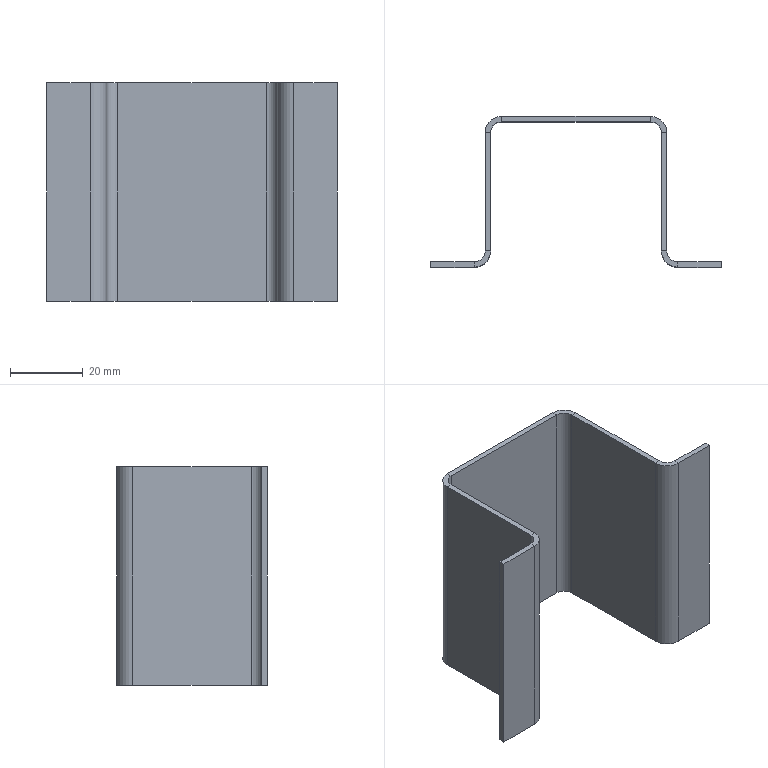Part | SolidWorks | features BaseBody 1 | 1 solid | 38 faces | box 80 x 41.5 x 60 mm | volume 13821 mm3 | plane 30 | cylinder 8 | commonest cylinder face diameters 6 x4 9 x4
STEP:
#1=CARTESIAN_POINT('',(68.,-1.5,-30.));
#2=VERTEX_POINT('',#1);
#3=CARTESIAN_POINT('',(80.,-1.5,-30.));
#4=VERTEX_POINT('',#3);
#5=CARTESIAN_POINT('',(65.,-1.5,-30.));
#6=DIRECTION('',(1.,0.,0.));
#7=VECTOR('',#6,1000.);
#8=LINE('',#5,#7);
#9=EDGE_CURVE('',#2,#4,#8,.T.);
#10=ORIENTED_EDGE('',*,*,#9,.F.);
#11=CARTESIAN_POINT('',(68.,0.,-30.));
#12=VERTEX_POINT('',#11);
#13=CARTESIAN_POINT('',(68.,-1.5,-30.));
#14=DIRECTION('',(0.,1.,0.));
#15=VECTOR('',#14,1000.);
#16=LINE('',#13,#15);
#17=EDGE_CURVE('',#2,#12,#16,.T.);
#18=ORIENTED_EDGE('',*,*,#17,.T.);
#19=CARTESIAN_POINT('',(80.,0.,-30.));
#20=VERTEX_POINT('',#19);
#21=CARTESIAN_POINT('',(65.,0.,-30.));
#22=DIRECTION('',(1.,0.,0.));
#23=VECTOR('',#22,1000.);
#24=LINE('',#21,#23);
#25=EDGE_CURVE('',#12,#20,#24,.T.);
#26=ORIENTED_EDGE('',*,*,#25,.T.);
#27=CARTESIAN_POINT('',(80.,0.,-30.));
#28=DIRECTION('',(0.,-1.,0.));
#29=VECTOR('',#28,1000.);
#30=LINE('',#27,#29);
#31=EDGE_CURVE('',#20,#4,#30,.T.);
#32=ORIENTED_EDGE('',*,*,#31,.T.);
#33=EDGE_LOOP('',(#10,#18,#26,#32));
#34=FACE_OUTER_BOUND('',#33,.T.);
#35=CARTESIAN_POINT('',(68.,3.,-30.));
#36=DIRECTION('',(0.,0.,-1.));
#37=DIRECTION('',(0.,-1.,0.));
#38=AXIS2_PLACEMENT_3D('',#35,#36,#37);
#39=PLANE('',#38);
#40=ADVANCED_FACE('',(#34),#39,.T.);
#41=CARTESIAN_POINT('',(0.,-1.5,30.));
#42=VERTEX_POINT('',#41);
#43=CARTESIAN_POINT('',(12.,-1.5,30.));
#44=VERTEX_POINT('',#43);
#45=CARTESIAN_POINT('',(0.,-1.5,30.));
#46=DIRECTION('',(1.,0.,0.));
#47=VECTOR('',#46,1000.);
#48=LINE('',#45,#47);
#49=EDGE_CURVE('',#42,#44,#48,.T.);
#50=ORIENTED_EDGE('',*,*,#49,.T.);
#51=CARTESIAN_POINT('',(12.,0.,30.));
#52=VERTEX_POINT('',#51);
#53=CARTESIAN_POINT('',(12.,-1.5,30.));
#54=DIRECTION('',(0.,1.,0.));
#55=VECTOR('',#54,1000.);
#56=LINE('',#53,#55);
#57=EDGE_CURVE('',#44,#52,#56,.T.);
#58=ORIENTED_EDGE('',*,*,#57,.T.);
#59=CARTESIAN_POINT('',(0.,0.,30.));
#60=VERTEX_POINT('',#59);
#61=CARTESIAN_POINT('',(0.,0.,30.));
#62=DIRECTION('',(1.,0.,0.));
#63=VECTOR('',#62,1000.);
#64=LINE('',#61,#63);
#65=EDGE_CURVE('',#60,#52,#64,.T.);
#66=ORIENTED_EDGE('',*,*,#65,.F.);
#67=CARTESIAN_POINT('',(0.,-1.5,30.));
#68=DIRECTION('',(0.,1.,0.));
#69=VECTOR('',#68,1000.);
#70=LINE('',#67,#69);
#71=EDGE_CURVE('',#42,#60,#70,.T.);
#72=ORIENTED_EDGE('',*,*,#71,.F.);
#73=EDGE_LOOP('',(#50,#58,#66,#72));
#74=FACE_OUTER_BOUND('',#73,.T.);
#75=CARTESIAN_POINT('',(68.,3.,30.));
#76=DIRECTION('',(0.,0.,-1.));
#77=DIRECTION('',(0.,-1.,0.));
#78=AXIS2_PLACEMENT_3D('',#75,#76,#77);
#79=PLANE('',#78);
#80=ADVANCED_FACE('',(#74),#79,.F.);
#81=CARTESIAN_POINT('',(63.5,3.,-30.));
#82=VERTEX_POINT('',#81);
#83=CARTESIAN_POINT('',(68.,3.,-30.));
#84=DIRECTION('',(0.,0.,1.));
#85=DIRECTION('',(1.,0.,0.));
#86=AXIS2_PLACEMENT_3D('',#83,#84,#85);
#87=CIRCLE('',#86,4.5);
#88=EDGE_CURVE('',#82,#2,#87,.T.);
#89=ORIENTED_EDGE('',*,*,#88,.T.);
#90=CARTESIAN_POINT('',(68.,-1.5,30.));
#91=VERTEX_POINT('',#90);
#92=CARTESIAN_POINT('',(68.,-1.5,30.));
#93=DIRECTION('',(0.,0.,-1.));
#94=VECTOR('',#93,1000.);
#95=LINE('',#92,#94);
#96=EDGE_CURVE('',#91,#2,#95,.T.);
#97=ORIENTED_EDGE('',*,*,#96,.F.);
#98=CARTESIAN_POINT('',(63.5,3.,30.));
#99=VERTEX_POINT('',#98);
#100=CARTESIAN_POINT('',(68.,3.,30.));
#101=DIRECTION('',(0.,0.,1.));
#102=DIRECTION('',(1.,0.,0.));
#103=AXIS2_PLACEMENT_3D('',#100,#101,#102);
#104=CIRCLE('',#103,4.5);
#105=EDGE_CURVE('',#99,#91,#104,.T.);
#106=ORIENTED_EDGE('',*,*,#105,.F.);
#107=CARTESIAN_POINT('',(63.5,3.,30.));
#108=DIRECTION('',(0.,0.,-1.));
#109=VECTOR('',#108,1000.);
#110=LINE('',#107,#109);
#111=EDGE_CURVE('',#99,#82,#110,.T.);
#112=ORIENTED_EDGE('',*,*,#111,.T.);
#113=EDGE_LOOP('',(#89,#97,#106,#112));
#114=FACE_OUTER_BOUND('',#113,.T.);
#115=CARTESIAN_POINT('',(68.,3.,30.));
#116=DIRECTION('',(0.,0.,-1.));
#117=DIRECTION('',(-1.,0.,0.));
#118=AXIS2_PLACEMENT_3D('',#115,#116,#117);
#119=CYLINDRICAL_SURFACE('',#118,4.5);
#120=ADVANCED_FACE('',(#114),#119,.T.);
#121=CARTESIAN_POINT('',(63.5,35.5,-30.));
#122=VERTEX_POINT('',#121);
#123=CARTESIAN_POINT('',(63.5,40.,-30.));
#124=DIRECTION('',(0.,-1.,0.));
#125=VECTOR('',#124,1000.);
#126=LINE('',#123,#125);
#127=EDGE_CURVE('',#122,#82,#126,.T.);
#128=ORIENTED_EDGE('',*,*,#127,.T.);
#129=ORIENTED_EDGE('',*,*,#111,.F.);
#130=CARTESIAN_POINT('',(63.5,35.5,30.));
#131=VERTEX_POINT('',#130);
#132=CARTESIAN_POINT('',(63.5,40.,30.));
#133=DIRECTION('',(0.,-1.,0.));
#134=VECTOR('',#133,1000.);
#135=LINE('',#132,#134);
#136=EDGE_CURVE('',#131,#99,#135,.T.);
#137=ORIENTED_EDGE('',*,*,#136,.F.);
#138=CARTESIAN_POINT('',(63.5,35.5,30.));
#139=DIRECTION('',(0.,0.,-1.));
#140=VECTOR('',#139,1000.);
#141=LINE('',#138,#140);
#142=EDGE_CURVE('',#131,#122,#141,.T.);
#143=ORIENTED_EDGE('',*,*,#142,.T.);
#144=EDGE_LOOP('',(#128,#129,#137,#143));
#145=FACE_OUTER_BOUND('',#144,.T.);
#146=CARTESIAN_POINT('',(63.5,40.,30.));
#147=DIRECTION('',(1.,0.,0.));
#148=DIRECTION('',(0.,1.,0.));
#149=AXIS2_PLACEMENT_3D('',#146,#147,#148);
#150=PLANE('',#149);
#151=ADVANCED_FACE('',(#145),#150,.F.);
#152=CARTESIAN_POINT('',(60.5,38.5,-30.));
#153=VERTEX_POINT('',#152);
#154=CARTESIAN_POINT('',(60.5,35.5,-30.));
#155=DIRECTION('',(0.,0.,-1.));
#156=DIRECTION('',(1.,0.,0.));
#157=AXIS2_PLACEMENT_3D('',#154,#155,#156);
#158=CIRCLE('',#157,3.);
#159=EDGE_CURVE('',#153,#122,#158,.T.);
#160=ORIENTED_EDGE('',*,*,#159,.T.);
#161=ORIENTED_EDGE('',*,*,#142,.F.);
#162=CARTESIAN_POINT('',(60.5,38.5,30.));
#163=VERTEX_POINT('',#162);
#164=CARTESIAN_POINT('',(60.5,35.5,30.));
#165=DIRECTION('',(0.,0.,-1.));
#166=DIRECTION('',(1.,0.,0.));
#167=AXIS2_PLACEMENT_3D('',#164,#165,#166);
#168=CIRCLE('',#167,3.);
#169=EDGE_CURVE('',#163,#131,#168,.T.);
#170=ORIENTED_EDGE('',*,*,#169,.F.);
#171=CARTESIAN_POINT('',(60.5,38.5,30.));
#172=DIRECTION('',(0.,0.,-1.));
#173=VECTOR('',#172,1000.);
#174=LINE('',#171,#173);
#175=EDGE_CURVE('',#163,#153,#174,.T.);
#176=ORIENTED_EDGE('',*,*,#175,.T.);
#177=EDGE_LOOP('',(#160,#161,#170,#176));
#178=FACE_OUTER_BOUND('',#177,.T.);
#179=CARTESIAN_POINT('',(60.5,35.5,30.));
#180=DIRECTION('',(0.,0.,-1.));
#181=DIRECTION('',(-1.,0.,0.));
#182=AXIS2_PLACEMENT_3D('',#179,#180,#181);
#183=CYLINDRICAL_SURFACE('',#182,3.);
#184=ADVANCED_FACE('',(#178),#183,.F.);
#185=CARTESIAN_POINT('',(19.5,38.5,-30.));
#186=VERTEX_POINT('',#185);
#187=CARTESIAN_POINT('',(15.,38.5,-30.));
#188=DIRECTION('',(1.,0.,0.));
#189=VECTOR('',#188,1000.);
#190=LINE('',#187,#189);
#191=EDGE_CURVE('',#186,#153,#190,.T.);
#192=ORIENTED_EDGE('',*,*,#191,.T.);
#193=ORIENTED_EDGE('',*,*,#175,.F.);
#194=CARTESIAN_POINT('',(19.5,38.5,30.));
#195=VERTEX_POINT('',#194);
#196=CARTESIAN_POINT('',(15.,38.5,30.));
#197=DIRECTION('',(1.,0.,0.));
#198=VECTOR('',#197,1000.);
#199=LINE('',#196,#198);
#200=EDGE_CURVE('',#195,#163,#199,.T.);
#201=ORIENTED_EDGE('',*,*,#200,.F.);
#202=CARTESIAN_POINT('',(19.5,38.5,30.));
#203=DIRECTION('',(0.,0.,-1.));
#204=VECTOR('',#203,1000.);
#205=LINE('',#202,#204);
#206=EDGE_CURVE('',#195,#186,#205,.T.);
#207=ORIENTED_EDGE('',*,*,#206,.T.);
#208=EDGE_LOOP('',(#192,#193,#201,#207));
#209=FACE_OUTER_BOUND('',#208,.T.);
#210=CARTESIAN_POINT('',(15.,38.5,30.));
#211=DIRECTION('',(0.,1.,0.));
#212=DIRECTION('',(1.,0.,0.));
#213=AXIS2_PLACEMENT_3D('',#210,#211,#212);
#214=PLANE('',#213);
#215=ADVANCED_FACE('',(#209),#214,.F.);
#216=CARTESIAN_POINT('',(16.5,35.5,-30.));
#217=VERTEX_POINT('',#216);
#218=CARTESIAN_POINT('',(19.5,35.5,-30.));
#219=DIRECTION('',(0.,0.,-1.));
#220=DIRECTION('',(1.,0.,0.));
#221=AXIS2_PLACEMENT_3D('',#218,#219,#220);
#222=CIRCLE('',#221,3.);
#223=EDGE_CURVE('',#217,#186,#222,.T.);
#224=ORIENTED_EDGE('',*,*,#223,.T.);
#225=ORIENTED_EDGE('',*,*,#206,.F.);
#226=CARTESIAN_POINT('',(16.5,35.5,30.));
#227=VERTEX_POINT('',#226);
#228=CARTESIAN_POINT('',(19.5,35.5,30.));
#229=DIRECTION('',(0.,0.,-1.));
#230=DIRECTION('',(1.,0.,0.));
#231=AXIS2_PLACEMENT_3D('',#228,#229,#230);
#232=CIRCLE('',#231,3.);
#233=EDGE_CURVE('',#227,#195,#232,.T.);
#234=ORIENTED_EDGE('',*,*,#233,.F.);
#235=CARTESIAN_POINT('',(16.5,35.5,30.));
#236=DIRECTION('',(0.,0.,-1.));
#237=VECTOR('',#236,1000.);
#238=LINE('',#235,#237);
#239=EDGE_CURVE('',#227,#217,#238,.T.);
#240=ORIENTED_EDGE('',*,*,#239,.T.);
#241=EDGE_LOOP('',(#224,#225,#234,#240));
#242=FACE_OUTER_BOUND('',#241,.T.);
#243=CARTESIAN_POINT('',(19.5,35.5,30.));
#244=DIRECTION('',(0.,0.,-1.));
#245=DIRECTION('',(-1.,0.,0.));
#246=AXIS2_PLACEMENT_3D('',#243,#244,#245);
#247=CYLINDRICAL_SURFACE('',#246,3.);
#248=ADVANCED_FACE('',(#242),#247,.F.);
#249=CARTESIAN_POINT('',(16.5,3.,-30.));
#250=VERTEX_POINT('',#249);
#251=CARTESIAN_POINT('',(16.5,0.,-30.));
#252=DIRECTION('',(0.,1.,0.));
#253=VECTOR('',#252,1000.);
#254=LINE('',#251,#253);
#255=EDGE_CURVE('',#250,#217,#254,.T.);
#256=ORIENTED_EDGE('',*,*,#255,.T.);
#257=ORIENTED_EDGE('',*,*,#239,.F.);
#258=CARTESIAN_POINT('',(16.5,3.,30.));
#259=VERTEX_POINT('',#258);
#260=CARTESIAN_POINT('',(16.5,0.,30.));
#261=DIRECTION('',(0.,1.,0.));
#262=VECTOR('',#261,1000.);
#263=LINE('',#260,#262);
#264=EDGE_CURVE('',#259,#227,#263,.T.);
#265=ORIENTED_EDGE('',*,*,#264,.F.);
#266=CARTESIAN_POINT('',(16.5,3.,30.));
#267=DIRECTION('',(0.,0.,-1.));
#268=VECTOR('',#267,1000.);
#269=LINE('',#266,#268);
#270=EDGE_CURVE('',#259,#250,#269,.T.);
#271=ORIENTED_EDGE('',*,*,#270,.T.);
#272=EDGE_LOOP('',(#256,#257,#265,#271));
#273=FACE_OUTER_BOUND('',#272,.T.);
#274=CARTESIAN_POINT('',(16.5,0.,30.));
#275=DIRECTION('',(-1.,0.,0.));
#276=DIRECTION('',(0.,0.,1.));
#277=AXIS2_PLACEMENT_3D('',#274,#275,#276);
#278=PLANE('',#277);
#279=ADVANCED_FACE('',(#273),#278,.F.);
#280=CARTESIAN_POINT('',(12.,-1.5,-30.));
#281=VERTEX_POINT('',#280);
#282=CARTESIAN_POINT('',(12.,3.,-30.));
#283=DIRECTION('',(0.,0.,1.));
#284=DIRECTION('',(1.,0.,0.));
#285=AXIS2_PLACEMENT_3D('',#282,#283,#284);
#286=CIRCLE('',#285,4.5);
#287=EDGE_CURVE('',#281,#250,#286,.T.);
#288=ORIENTED_EDGE('',*,*,#287,.T.);
#289=ORIENTED_EDGE('',*,*,#270,.F.);
#290=CARTESIAN_POINT('',(12.,3.,30.));
#291=DIRECTION('',(0.,0.,1.));
#292=DIRECTION('',(1.,0.,0.));
#293=AXIS2_PLACEMENT_3D('',#290,#291,#292);
#294=CIRCLE('',#293,4.5);
#295=EDGE_CURVE('',#44,#259,#294,.T.);
#296=ORIENTED_EDGE('',*,*,#295,.F.);
#297=CARTESIAN_POINT('',(12.,-1.5,30.));
#298=DIRECTION('',(0.,0.,-1.));
#299=VECTOR('',#298,1000.);
#300=LINE('',#297,#299);
#301=EDGE_CURVE('',#44,#281,#300,.T.);
#302=ORIENTED_EDGE('',*,*,#301,.T.);
#303=EDGE_LOOP('',(#288,#289,#296,#302));
#304=FACE_OUTER_BOUND('',#303,.T.);
#305=CARTESIAN_POINT('',(12.,3.,30.));
#306=DIRECTION('',(0.,0.,-1.));
#307=DIRECTION('',(-1.,0.,0.));
#308=AXIS2_PLACEMENT_3D('',#305,#306,#307);
#309=CYLINDRICAL_SURFACE('',#308,4.5);
#310=ADVANCED_FACE('',(#304),#309,.T.);
#311=CARTESIAN_POINT('',(0.,-1.5,-30.));
#312=VERTEX_POINT('',#311);
#313=CARTESIAN_POINT('',(0.,-1.5,-30.));
#314=DIRECTION('',(1.,0.,0.));
#315=VECTOR('',#314,1000.);
#316=LINE('',#313,#315);
#317=EDGE_CURVE('',#312,#281,#316,.T.);
#318=ORIENTED_EDGE('',*,*,#317,.T.);
#319=ORIENTED_EDGE('',*,*,#301,.F.);
#320=ORIENTED_EDGE('',*,*,#49,.F.);
#321=CARTESIAN_POINT('',(0.,-1.5,30.));
#322=DIRECTION('',(0.,0.,-1.));
#323=VECTOR('',#322,1000.);
#324=LINE('',#321,#323);
#325=EDGE_CURVE('',#42,#312,#324,.T.);
#326=ORIENTED_EDGE('',*,*,#325,.T.);
#327=EDGE_LOOP('',(#318,#319,#320,#326));
#328=FACE_OUTER_BOUND('',#327,.T.);
#329=CARTESIAN_POINT('',(0.,-1.5,30.));
#330=DIRECTION('',(0.,1.,0.));
#331=DIRECTION('',(1.,0.,0.));
#332=AXIS2_PLACEMENT_3D('',#329,#330,#331);
#333=PLANE('',#332);
#334=ADVANCED_FACE('',(#328),#333,.F.);
#335=CARTESIAN_POINT('',(0.,0.,-30.));
#336=VERTEX_POINT('',#335);
#337=CARTESIAN_POINT('',(0.,-1.5,-30.));
#338=DIRECTION('',(0.,1.,0.));
#339=VECTOR('',#338,1000.);
#340=LINE('',#337,#339);
#341=EDGE_CURVE('',#312,#336,#340,.T.);
#342=ORIENTED_EDGE('',*,*,#341,.F.);
#343=ORIENTED_EDGE('',*,*,#325,.F.);
#344=ORIENTED_EDGE('',*,*,#71,.T.);
#345=CARTESIAN_POINT('',(0.,0.,30.));
#346=DIRECTION('',(0.,0.,-1.));
#347=VECTOR('',#346,1000.);
#348=LINE('',#345,#347);
#349=EDGE_CURVE('',#60,#336,#348,.T.);
#350=ORIENTED_EDGE('',*,*,#349,.T.);
#351=EDGE_LOOP('',(#342,#343,#344,#350));
#352=FACE_OUTER_BOUND('',#351,.T.);
#353=CARTESIAN_POINT('',(0.,-1.5,30.));
#354=DIRECTION('',(-1.,0.,0.));
#355=DIRECTION('',(0.,0.,1.));
#356=AXIS2_PLACEMENT_3D('',#353,#354,#355);
#357=PLANE('',#356);
#358=ADVANCED_FACE('',(#352),#357,.T.);
#359=CARTESIAN_POINT('',(12.,0.,-30.));
#360=VERTEX_POINT('',#359);
#361=CARTESIAN_POINT('',(0.,0.,-30.));
#362=DIRECTION('',(1.,0.,0.));
#363=VECTOR('',#362,1000.);
#364=LINE('',#361,#363);
#365=EDGE_CURVE('',#336,#360,#364,.T.);
#366=ORIENTED_EDGE('',*,*,#365,.F.);
#367=ORIENTED_EDGE('',*,*,#349,.F.);
#368=ORIENTED_EDGE('',*,*,#65,.T.);
#369=CARTESIAN_POINT('',(12.,0.,30.));
#370=DIRECTION('',(0.,0.,-1.));
#371=VECTOR('',#370,1000.);
#372=LINE('',#369,#371);
#373=EDGE_CURVE('',#52,#360,#372,.T.);
#374=ORIENTED_EDGE('',*,*,#373,.T.);
#375=EDGE_LOOP('',(#366,#367,#368,#374));
#376=FACE_OUTER_BOUND('',#375,.T.);
#377=CARTESIAN_POINT('',(0.,0.,30.));
#378=DIRECTION('',(0.,1.,0.));
#379=DIRECTION('',(1.,0.,0.));
#380=AXIS2_PLACEMENT_3D('',#377,#378,#379);
#381=PLANE('',#380);
#382=ADVANCED_FACE('',(#376),#381,.T.);
#383=CARTESIAN_POINT('',(15.,3.,-30.));
#384=VERTEX_POINT('',#383);
#385=CARTESIAN_POINT('',(12.,3.,-30.));
#386=DIRECTION('',(0.,0.,1.));
#387=DIRECTION('',(-1.,0.,0.));
#388=AXIS2_PLACEMENT_3D('',#385,#386,#387);
#389=CIRCLE('',#388,3.);
#390=EDGE_CURVE('',#360,#384,#389,.T.);
#391=ORIENTED_EDGE('',*,*,#390,.F.);
#392=ORIENTED_EDGE('',*,*,#373,.F.);
#393=CARTESIAN_POINT('',(15.,3.,30.));
#394=VERTEX_POINT('',#393);
#395=CARTESIAN_POINT('',(12.,3.,30.));
#396=DIRECTION('',(0.,0.,1.));
#397=DIRECTION('',(-1.,0.,0.));
#398=AXIS2_PLACEMENT_3D('',#395,#396,#397);
#399=CIRCLE('',#398,3.);
#400=EDGE_CURVE('',#52,#394,#399,.T.);
#401=ORIENTED_EDGE('',*,*,#400,.T.);
#402=CARTESIAN_POINT('',(15.,3.,30.));
#403=DIRECTION('',(0.,0.,-1.));
#404=VECTOR('',#403,1000.);
#405=LINE('',#402,#404);
#406=EDGE_CURVE('',#394,#384,#405,.T.);
#407=ORIENTED_EDGE('',*,*,#406,.T.);
#408=EDGE_LOOP('',(#391,#392,#401,#407));
#409=FACE_OUTER_BOUND('',#408,.T.);
#410=CARTESIAN_POINT('',(12.,3.,30.));
#411=DIRECTION('',(0.,0.,-1.));
#412=DIRECTION('',(-1.,0.,0.));
#413=AXIS2_PLACEMENT_3D('',#410,#411,#412);
#414=CYLINDRICAL_SURFACE('',#413,3.);
#415=ADVANCED_FACE('',(#409),#414,.F.);
#416=CARTESIAN_POINT('',(15.,35.5,-30.));
#417=VERTEX_POINT('',#416);
#418=CARTESIAN_POINT('',(15.,0.,-30.));
#419=DIRECTION('',(0.,1.,0.));
#420=VECTOR('',#419,1000.);
#421=LINE('',#418,#420);
#422=EDGE_CURVE('',#384,#417,#421,.T.);
#423=ORIENTED_EDGE('',*,*,#422,.F.);
#424=ORIENTED_EDGE('',*,*,#406,.F.);
#425=CARTESIAN_POINT('',(15.,35.5,30.));
#426=VERTEX_POINT('',#425);
#427=CARTESIAN_POINT('',(15.,0.,30.));
#428=DIRECTION('',(0.,1.,0.));
#429=VECTOR('',#428,1000.);
#430=LINE('',#427,#429);
#431=EDGE_CURVE('',#394,#426,#430,.T.);
#432=ORIENTED_EDGE('',*,*,#431,.T.);
#433=CARTESIAN_POINT('',(15.,35.5,30.));
#434=DIRECTION('',(0.,0.,-1.));
#435=VECTOR('',#434,1000.);
#436=LINE('',#433,#435);
#437=EDGE_CURVE('',#426,#417,#436,.T.);
#438=ORIENTED_EDGE('',*,*,#437,.T.);
#439=EDGE_LOOP('',(#423,#424,#432,#438));
#440=FACE_OUTER_BOUND('',#439,.T.);
#441=CARTESIAN_POINT('',(15.,0.,30.));
#442=DIRECTION('',(-1.,0.,0.));
#443=DIRECTION('',(0.,0.,1.));
#444=AXIS2_PLACEMENT_3D('',#441,#442,#443);
#445=PLANE('',#444);
#446=ADVANCED_FACE('',(#440),#445,.T.);
#447=CARTESIAN_POINT('',(19.5,40.,-30.));
#448=VERTEX_POINT('',#447);
#449=CARTESIAN_POINT('',(19.5,35.5,-30.));
#450=DIRECTION('',(0.,0.,-1.));
#451=DIRECTION('',(1.,0.,0.));
#452=AXIS2_PLACEMENT_3D('',#449,#450,#451);
#453=CIRCLE('',#452,4.5);
#454=EDGE_CURVE('',#417,#448,#453,.T.);
#455=ORIENTED_EDGE('',*,*,#454,.F.);
#456=ORIENTED_EDGE('',*,*,#437,.F.);
#457=CARTESIAN_POINT('',(19.5,40.,30.));
#458=VERTEX_POINT('',#457);
#459=CARTESIAN_POINT('',(19.5,35.5,30.));
#460=DIRECTION('',(0.,0.,-1.));
#461=DIRECTION('',(1.,0.,0.));
#462=AXIS2_PLACEMENT_3D('',#459,#460,#461);
#463=CIRCLE('',#462,4.5);
#464=EDGE_CURVE('',#426,#458,#463,.T.);
#465=ORIENTED_EDGE('',*,*,#464,.T.);
#466=CARTESIAN_POINT('',(19.5,40.,30.));
#467=DIRECTION('',(0.,0.,-1.));
#468=VECTOR('',#467,1000.);
#469=LINE('',#466,#468);
#470=EDGE_CURVE('',#458,#448,#469,.T.);
#471=ORIENTED_EDGE('',*,*,#470,.T.);
#472=EDGE_LOOP('',(#455,#456,#465,#471));
#473=FACE_OUTER_BOUND('',#472,.T.);
#474=CARTESIAN_POINT('',(19.5,35.5,30.));
#475=DIRECTION('',(0.,0.,-1.));
#476=DIRECTION('',(-1.,0.,0.));
#477=AXIS2_PLACEMENT_3D('',#474,#475,#476);
#478=CYLINDRICAL_SURFACE('',#477,4.5);
#479=ADVANCED_FACE('',(#473),#478,.T.);
#480=CARTESIAN_POINT('',(60.5,40.,-30.));
#481=VERTEX_POINT('',#480);
#482=CARTESIAN_POINT('',(15.,40.,-30.));
#483=DIRECTION('',(1.,0.,0.));
#484=VECTOR('',#483,1000.);
#485=LINE('',#482,#484);
#486=EDGE_CURVE('',#448,#481,#485,.T.);
#487=ORIENTED_EDGE('',*,*,#486,.F.);
#488=ORIENTED_EDGE('',*,*,#470,.F.);
#489=CARTESIAN_POINT('',(60.5,40.,30.));
#490=VERTEX_POINT('',#489);
#491=CARTESIAN_POINT('',(15.,40.,30.));
#492=DIRECTION('',(1.,0.,0.));
#493=VECTOR('',#492,1000.);
#494=LINE('',#491,#493);
#495=EDGE_CURVE('',#458,#490,#494,.T.);
#496=ORIENTED_EDGE('',*,*,#495,.T.);
#497=CARTESIAN_POINT('',(60.5,40.,30.));
#498=DIRECTION('',(0.,0.,-1.));
#499=VECTOR('',#498,1000.);
#500=LINE('',#497,#499);
#501=EDGE_CURVE('',#490,#481,#500,.T.);
#502=ORIENTED_EDGE('',*,*,#501,.T.);
#503=EDGE_LOOP('',(#487,#488,#496,#502));
#504=FACE_OUTER_BOUND('',#503,.T.);
#505=CARTESIAN_POINT('',(15.,40.,30.));
#506=DIRECTION('',(0.,1.,0.));
#507=DIRECTION('',(1.,0.,0.));
#508=AXIS2_PLACEMENT_3D('',#505,#506,#507);
#509=PLANE('',#508);
#510=ADVANCED_FACE('',(#504),#509,.T.);
#511=CARTESIAN_POINT('',(65.,35.5,-30.));
#512=VERTEX_POINT('',#511);
#513=CARTESIAN_POINT('',(60.5,35.5,-30.));
#514=DIRECTION('',(0.,0.,-1.));
#515=DIRECTION('',(1.,0.,0.));
#516=AXIS2_PLACEMENT_3D('',#513,#514,#515);
#517=CIRCLE('',#516,4.5);
#518=EDGE_CURVE('',#481,#512,#517,.T.);
#519=ORIENTED_EDGE('',*,*,#518,.F.);
#520=ORIENTED_EDGE('',*,*,#501,.F.);
#521=CARTESIAN_POINT('',(65.,35.5,30.));
#522=VERTEX_POINT('',#521);
#523=CARTESIAN_POINT('',(60.5,35.5,30.));
#524=DIRECTION('',(0.,0.,-1.));
#525=DIRECTION('',(1.,0.,0.));
#526=AXIS2_PLACEMENT_3D('',#523,#524,#525);
#527=CIRCLE('',#526,4.5);
#528=EDGE_CURVE('',#490,#522,#527,.T.);
#529=ORIENTED_EDGE('',*,*,#528,.T.);
#530=CARTESIAN_POINT('',(65.,35.5,30.));
#531=DIRECTION('',(0.,0.,-1.));
#532=VECTOR('',#531,1000.);
#533=LINE('',#530,#532);
#534=EDGE_CURVE('',#522,#512,#533,.T.);
#535=ORIENTED_EDGE('',*,*,#534,.T.);
#536=EDGE_LOOP('',(#519,#520,#529,#535));
#537=FACE_OUTER_BOUND('',#536,.T.);
#538=CARTESIAN_POINT('',(60.5,35.5,30.));
#539=DIRECTION('',(0.,0.,-1.));
#540=DIRECTION('',(-1.,0.,0.));
#541=AXIS2_PLACEMENT_3D('',#538,#539,#540);
#542=CYLINDRICAL_SURFACE('',#541,4.5);
#543=ADVANCED_FACE('',(#537),#542,.T.);
#544=CARTESIAN_POINT('',(65.,3.,-30.));
#545=VERTEX_POINT('',#544);
#546=CARTESIAN_POINT('',(65.,40.,-30.));
#547=DIRECTION('',(0.,-1.,0.));
#548=VECTOR('',#547,1000.);
#549=LINE('',#546,#548);
#550=EDGE_CURVE('',#512,#545,#549,.T.);
#551=ORIENTED_EDGE('',*,*,#550,.F.);
#552=ORIENTED_EDGE('',*,*,#534,.F.);
#553=CARTESIAN_POINT('',(65.,3.,30.));
#554=VERTEX_POINT('',#553);
#555=CARTESIAN_POINT('',(65.,40.,30.));
#556=DIRECTION('',(0.,-1.,0.));
#557=VECTOR('',#556,1000.);
#558=LINE('',#555,#557);
#559=EDGE_CURVE('',#522,#554,#558,.T.);
#560=ORIENTED_EDGE('',*,*,#559,.T.);
#561=CARTESIAN_POINT('',(65.,3.,30.));
#562=DIRECTION('',(0.,0.,-1.));
#563=VECTOR('',#562,1000.);
#564=LINE('',#561,#563);
#565=EDGE_CURVE('',#554,#545,#564,.T.);
#566=ORIENTED_EDGE('',*,*,#565,.T.);
#567=EDGE_LOOP('',(#551,#552,#560,#566));
#568=FACE_OUTER_BOUND('',#567,.T.);
#569=CARTESIAN_POINT('',(65.,40.,30.));
#570=DIRECTION('',(1.,0.,0.));
#571=DIRECTION('',(0.,1.,0.));
#572=AXIS2_PLACEMENT_3D('',#569,#570,#571);
#573=PLANE('',#572);
#574=ADVANCED_FACE('',(#568),#573,.T.);
#575=CARTESIAN_POINT('',(68.,3.,-30.));
#576=DIRECTION('',(0.,0.,1.));
#577=DIRECTION('',(-1.,0.,0.));
#578=AXIS2_PLACEMENT_3D('',#575,#576,#577);
#579=CIRCLE('',#578,3.);
#580=EDGE_CURVE('',#545,#12,#579,.T.);
#581=ORIENTED_EDGE('',*,*,#580,.F.);
#582=ORIENTED_EDGE('',*,*,#565,.F.);
#583=CARTESIAN_POINT('',(68.,0.,30.));
#584=VERTEX_POINT('',#583);
#585=CARTESIAN_POINT('',(68.,3.,30.));
#586=DIRECTION('',(0.,0.,1.));
#587=DIRECTION('',(-1.,0.,0.));
#588=AXIS2_PLACEMENT_3D('',#585,#586,#587);
#589=CIRCLE('',#588,3.);
#590=EDGE_CURVE('',#554,#584,#589,.T.);
#591=ORIENTED_EDGE('',*,*,#590,.T.);
#592=CARTESIAN_POINT('',(68.,0.,30.));
#593=DIRECTION('',(0.,0.,-1.));
#594=VECTOR('',#593,1000.);
#595=LINE('',#592,#594);
#596=EDGE_CURVE('',#584,#12,#595,.T.);
#597=ORIENTED_EDGE('',*,*,#596,.T.);
#598=EDGE_LOOP('',(#581,#582,#591,#597));
#599=FACE_OUTER_BOUND('',#598,.T.);
#600=CARTESIAN_POINT('',(68.,3.,30.));
#601=DIRECTION('',(0.,0.,-1.));
#602=DIRECTION('',(-1.,0.,0.));
#603=AXIS2_PLACEMENT_3D('',#600,#601,#602);
#604=CYLINDRICAL_SURFACE('',#603,3.);
#605=ADVANCED_FACE('',(#599),#604,.F.);
#606=ORIENTED_EDGE('',*,*,#25,.F.);
#607=ORIENTED_EDGE('',*,*,#596,.F.);
#608=CARTESIAN_POINT('',(80.,0.,30.));
#609=VERTEX_POINT('',#608);
#610=CARTESIAN_POINT('',(65.,0.,30.));
#611=DIRECTION('',(1.,0.,0.));
#612=VECTOR('',#611,1000.);
#613=LINE('',#610,#612);
#614=EDGE_CURVE('',#584,#609,#613,.T.);
#615=ORIENTED_EDGE('',*,*,#614,.T.);
#616=CARTESIAN_POINT('',(80.,0.,30.));
#617=DIRECTION('',(0.,0.,-1.));
#618=VECTOR('',#617,1000.);
#619=LINE('',#616,#618);
#620=EDGE_CURVE('',#609,#20,#619,.T.);
#621=ORIENTED_EDGE('',*,*,#620,.T.);
#622=EDGE_LOOP('',(#606,#607,#615,#621));
#623=FACE_OUTER_BOUND('',#622,.T.);
#624=CARTESIAN_POINT('',(65.,0.,30.));
#625=DIRECTION('',(0.,1.,0.));
#626=DIRECTION('',(1.,0.,0.));
#627=AXIS2_PLACEMENT_3D('',#624,#625,#626);
#628=PLANE('',#627);
#629=ADVANCED_FACE('',(#623),#628,.T.);
#630=ORIENTED_EDGE('',*,*,#31,.F.);
#631=ORIENTED_EDGE('',*,*,#620,.F.);
#632=CARTESIAN_POINT('',(80.,-1.5,30.));
#633=VERTEX_POINT('',#632);
#634=CARTESIAN_POINT('',(80.,0.,30.));
#635=DIRECTION('',(0.,-1.,0.));
#636=VECTOR('',#635,1000.);
#637=LINE('',#634,#636);
#638=EDGE_CURVE('',#609,#633,#637,.T.);
#639=ORIENTED_EDGE('',*,*,#638,.T.);
#640=CARTESIAN_POINT('',(80.,-1.5,30.));
#641=DIRECTION('',(0.,0.,-1.));
#642=VECTOR('',#641,1000.);
#643=LINE('',#640,#642);
#644=EDGE_CURVE('',#633,#4,#643,.T.);
#645=ORIENTED_EDGE('',*,*,#644,.T.);
#646=EDGE_LOOP('',(#630,#631,#639,#645));
#647=FACE_OUTER_BOUND('',#646,.T.);
#648=CARTESIAN_POINT('',(80.,0.,30.));
#649=DIRECTION('',(1.,0.,0.));
#650=DIRECTION('',(0.,1.,0.));
#651=AXIS2_PLACEMENT_3D('',#648,#649,#650);
#652=PLANE('',#651);
#653=ADVANCED_FACE('',(#647),#652,.T.);
#654=ORIENTED_EDGE('',*,*,#9,.T.);
#655=ORIENTED_EDGE('',*,*,#644,.F.);
#656=CARTESIAN_POINT('',(65.,-1.5,30.));
#657=DIRECTION('',(1.,0.,0.));
#658=VECTOR('',#657,1000.);
#659=LINE('',#656,#658);
#660=EDGE_CURVE('',#91,#633,#659,.T.);
#661=ORIENTED_EDGE('',*,*,#660,.F.);
#662=ORIENTED_EDGE('',*,*,#96,.T.);
#663=EDGE_LOOP('',(#654,#655,#661,#662));
#664=FACE_OUTER_BOUND('',#663,.T.);
#665=CARTESIAN_POINT('',(65.,-1.5,30.));
#666=DIRECTION('',(0.,1.,0.));
#667=DIRECTION('',(1.,0.,0.));
#668=AXIS2_PLACEMENT_3D('',#665,#666,#667);
#669=PLANE('',#668);
#670=ADVANCED_FACE('',(#664),#669,.F.);
#671=ORIENTED_EDGE('',*,*,#550,.T.);
#672=CARTESIAN_POINT('',(65.,3.,-30.));
#673=DIRECTION('',(-1.,0.,0.));
#674=VECTOR('',#673,1000.);
#675=LINE('',#672,#674);
#676=EDGE_CURVE('',#545,#82,#675,.T.);
#677=ORIENTED_EDGE('',*,*,#676,.T.);
#678=ORIENTED_EDGE('',*,*,#127,.F.);
#679=CARTESIAN_POINT('',(63.5,35.5,-30.));
#680=DIRECTION('',(1.,0.,0.));
#681=VECTOR('',#680,1000.);
#682=LINE('',#679,#681);
#683=EDGE_CURVE('',#122,#512,#682,.T.);
#684=ORIENTED_EDGE('',*,*,#683,.T.);
#685=EDGE_LOOP('',(#671,#677,#678,#684));
#686=FACE_OUTER_BOUND('',#685,.T.);
#687=CARTESIAN_POINT('',(68.,-1.5,-30.));
#688=DIRECTION('',(0.,0.,-1.));
#689=DIRECTION('',(0.,-1.,0.));
#690=AXIS2_PLACEMENT_3D('',#687,#688,#689);
#691=PLANE('',#690);
#692=ADVANCED_FACE('',(#686),#691,.T.);
#693=ORIENTED_EDGE('',*,*,#676,.F.);
#694=ORIENTED_EDGE('',*,*,#580,.T.);
#695=ORIENTED_EDGE('',*,*,#17,.F.);
#696=ORIENTED_EDGE('',*,*,#88,.F.);
#697=EDGE_LOOP('',(#693,#694,#695,#696));
#698=FACE_OUTER_BOUND('',#697,.T.);
#699=CARTESIAN_POINT('',(65.,3.,-30.));
#700=DIRECTION('',(0.,0.,-1.));
#701=DIRECTION('',(0.,-1.,0.));
#702=AXIS2_PLACEMENT_3D('',#699,#700,#701);
#703=PLANE('',#702);
#704=ADVANCED_FACE('',(#698),#703,.T.);
#705=ORIENTED_EDGE('',*,*,#614,.F.);
#706=CARTESIAN_POINT('',(68.,0.,30.));
#707=DIRECTION('',(0.,-1.,0.));
#708=VECTOR('',#707,1000.);
#709=LINE('',#706,#708);
#710=EDGE_CURVE('',#584,#91,#709,.T.);
#711=ORIENTED_EDGE('',*,*,#710,.T.);
#712=ORIENTED_EDGE('',*,*,#660,.T.);
#713=ORIENTED_EDGE('',*,*,#638,.F.);
#714=EDGE_LOOP('',(#705,#711,#712,#713));
#715=FACE_OUTER_BOUND('',#714,.T.);
#716=CARTESIAN_POINT('',(63.5,3.,30.));
#717=DIRECTION('',(0.,0.,1.));
#718=DIRECTION('',(1.,0.,0.));
#719=AXIS2_PLACEMENT_3D('',#716,#717,#718);
#720=PLANE('',#719);
#721=ADVANCED_FACE('',(#715),#720,.T.);
#722=ORIENTED_EDGE('',*,*,#710,.F.);
#723=ORIENTED_EDGE('',*,*,#590,.F.);
#724=CARTESIAN_POINT('',(63.5,3.,30.));
#725=DIRECTION('',(1.,0.,0.));
#726=VECTOR('',#725,1000.);
#727=LINE('',#724,#726);
#728=EDGE_CURVE('',#99,#554,#727,.T.);
#729=ORIENTED_EDGE('',*,*,#728,.F.);
#730=ORIENTED_EDGE('',*,*,#105,.T.);
#731=EDGE_LOOP('',(#722,#723,#729,#730));
#732=FACE_OUTER_BOUND('',#731,.T.);
#733=CARTESIAN_POINT('',(68.,0.,30.));
#734=DIRECTION('',(0.,0.,1.));
#735=DIRECTION('',(1.,0.,0.));
#736=AXIS2_PLACEMENT_3D('',#733,#734,#735);
#737=PLANE('',#736);
#738=ADVANCED_FACE('',(#732),#737,.T.);
#739=ORIENTED_EDGE('',*,*,#486,.T.);
#740=CARTESIAN_POINT('',(60.5,40.,-30.));
#741=DIRECTION('',(0.,-1.,0.));
#742=VECTOR('',#741,1000.);
#743=LINE('',#740,#742);
#744=EDGE_CURVE('',#481,#153,#743,.T.);
#745=ORIENTED_EDGE('',*,*,#744,.T.);
#746=ORIENTED_EDGE('',*,*,#191,.F.);
#747=CARTESIAN_POINT('',(19.5,38.5,-30.));
#748=DIRECTION('',(0.,1.,0.));
#749=VECTOR('',#748,1000.);
#750=LINE('',#747,#749);
#751=EDGE_CURVE('',#186,#448,#750,.T.);
#752=ORIENTED_EDGE('',*,*,#751,.T.);
#753=EDGE_LOOP('',(#739,#745,#746,#752));
#754=FACE_OUTER_BOUND('',#753,.T.);
#755=CARTESIAN_POINT('',(63.5,35.5,-30.));
#756=DIRECTION('',(0.,0.,-1.));
#757=DIRECTION('',(0.,-1.,0.));
#758=AXIS2_PLACEMENT_3D('',#755,#756,#757);
#759=PLANE('',#758);
#760=ADVANCED_FACE('',(#754),#759,.T.);
#761=ORIENTED_EDGE('',*,*,#744,.F.);
#762=ORIENTED_EDGE('',*,*,#518,.T.);
#763=ORIENTED_EDGE('',*,*,#683,.F.);
#764=ORIENTED_EDGE('',*,*,#159,.F.);
#765=EDGE_LOOP('',(#761,#762,#763,#764));
#766=FACE_OUTER_BOUND('',#765,.T.);
#767=CARTESIAN_POINT('',(60.5,40.,-30.));
#768=DIRECTION('',(0.,0.,-1.));
#769=DIRECTION('',(0.,-1.,0.));
#770=AXIS2_PLACEMENT_3D('',#767,#768,#769);
#771=PLANE('',#770);
#772=ADVANCED_FACE('',(#766),#771,.T.);
#773=ORIENTED_EDGE('',*,*,#559,.F.);
#774=CARTESIAN_POINT('',(65.,35.5,30.));
#775=DIRECTION('',(-1.,0.,0.));
#776=VECTOR('',#775,1000.);
#777=LINE('',#774,#776);
#778=EDGE_CURVE('',#522,#131,#777,.T.);
#779=ORIENTED_EDGE('',*,*,#778,.T.);
#780=ORIENTED_EDGE('',*,*,#136,.T.);
#781=ORIENTED_EDGE('',*,*,#728,.T.);
#782=EDGE_LOOP('',(#773,#779,#780,#781));
#783=FACE_OUTER_BOUND('',#782,.T.);
#784=CARTESIAN_POINT('',(60.5,38.5,30.));
#785=DIRECTION('',(0.,0.,1.));
#786=DIRECTION('',(1.,0.,0.));
#787=AXIS2_PLACEMENT_3D('',#784,#785,#786);
#788=PLANE('',#787);
#789=ADVANCED_FACE('',(#783),#788,.T.);
#790=ORIENTED_EDGE('',*,*,#778,.F.);
#791=ORIENTED_EDGE('',*,*,#528,.F.);
#792=CARTESIAN_POINT('',(60.5,38.5,30.));
#793=DIRECTION('',(0.,1.,0.));
#794=VECTOR('',#793,1000.);
#795=LINE('',#792,#794);
#796=EDGE_CURVE('',#163,#490,#795,.T.);
#797=ORIENTED_EDGE('',*,*,#796,.F.);
#798=ORIENTED_EDGE('',*,*,#169,.T.);
#799=EDGE_LOOP('',(#790,#791,#797,#798));
#800=FACE_OUTER_BOUND('',#799,.T.);
#801=CARTESIAN_POINT('',(65.,35.5,30.));
#802=DIRECTION('',(0.,0.,1.));
#803=DIRECTION('',(1.,0.,0.));
#804=AXIS2_PLACEMENT_3D('',#801,#802,#803);
#805=PLANE('',#804);
#806=ADVANCED_FACE('',(#800),#805,.T.);
#807=ORIENTED_EDGE('',*,*,#422,.T.);
#808=CARTESIAN_POINT('',(15.,35.5,-30.));
#809=DIRECTION('',(1.,0.,0.));
#810=VECTOR('',#809,1000.);
#811=LINE('',#808,#810);
#812=EDGE_CURVE('',#417,#217,#811,.T.);
#813=ORIENTED_EDGE('',*,*,#812,.T.);
#814=ORIENTED_EDGE('',*,*,#255,.F.);
#815=CARTESIAN_POINT('',(16.5,3.,-30.));
#816=DIRECTION('',(-1.,0.,0.));
#817=VECTOR('',#816,1000.);
#818=LINE('',#815,#817);
#819=EDGE_CURVE('',#250,#384,#818,.T.);
#820=ORIENTED_EDGE('',*,*,#819,.T.);
#821=EDGE_LOOP('',(#807,#813,#814,#820));
#822=FACE_OUTER_BOUND('',#821,.T.);
#823=CARTESIAN_POINT('',(19.5,38.5,-30.));
#824=DIRECTION('',(0.,0.,-1.));
#825=DIRECTION('',(0.,-1.,0.));
#826=AXIS2_PLACEMENT_3D('',#823,#824,#825);
#827=PLANE('',#826);
#828=ADVANCED_FACE('',(#822),#827,.T.);
#829=ORIENTED_EDGE('',*,*,#812,.F.);
#830=ORIENTED_EDGE('',*,*,#454,.T.);
#831=ORIENTED_EDGE('',*,*,#751,.F.);
#832=ORIENTED_EDGE('',*,*,#223,.F.);
#833=EDGE_LOOP('',(#829,#830,#831,#832));
#834=FACE_OUTER_BOUND('',#833,.T.);
#835=CARTESIAN_POINT('',(15.,35.5,-30.));
#836=DIRECTION('',(0.,0.,-1.));
#837=DIRECTION('',(0.,-1.,0.));
#838=AXIS2_PLACEMENT_3D('',#835,#836,#837);
#839=PLANE('',#838);
#840=ADVANCED_FACE('',(#834),#839,.T.);
#841=ORIENTED_EDGE('',*,*,#495,.F.);
#842=CARTESIAN_POINT('',(19.5,40.,30.));
#843=DIRECTION('',(0.,-1.,0.));
#844=VECTOR('',#843,1000.);
#845=LINE('',#842,#844);
#846=EDGE_CURVE('',#458,#195,#845,.T.);
#847=ORIENTED_EDGE('',*,*,#846,.T.);
#848=ORIENTED_EDGE('',*,*,#200,.T.);
#849=ORIENTED_EDGE('',*,*,#796,.T.);
#850=EDGE_LOOP('',(#841,#847,#848,#849));
#851=FACE_OUTER_BOUND('',#850,.T.);
#852=CARTESIAN_POINT('',(16.5,35.5,30.));
#853=DIRECTION('',(0.,0.,1.));
#854=DIRECTION('',(1.,0.,0.));
#855=AXIS2_PLACEMENT_3D('',#852,#853,#854);
#856=PLANE('',#855);
#857=ADVANCED_FACE('',(#851),#856,.T.);
#858=ORIENTED_EDGE('',*,*,#846,.F.);
#859=ORIENTED_EDGE('',*,*,#464,.F.);
#860=CARTESIAN_POINT('',(16.5,35.5,30.));
#861=DIRECTION('',(-1.,0.,0.));
#862=VECTOR('',#861,1000.);
#863=LINE('',#860,#862);
#864=EDGE_CURVE('',#227,#426,#863,.T.);
#865=ORIENTED_EDGE('',*,*,#864,.F.);
#866=ORIENTED_EDGE('',*,*,#233,.T.);
#867=EDGE_LOOP('',(#858,#859,#865,#866));
#868=FACE_OUTER_BOUND('',#867,.T.);
#869=CARTESIAN_POINT('',(19.5,40.,30.));
#870=DIRECTION('',(0.,0.,1.));
#871=DIRECTION('',(1.,0.,0.));
#872=AXIS2_PLACEMENT_3D('',#869,#870,#871);
#873=PLANE('',#872);
#874=ADVANCED_FACE('',(#868),#873,.T.);
#875=ORIENTED_EDGE('',*,*,#365,.T.);
#876=CARTESIAN_POINT('',(12.,0.,-30.));
#877=DIRECTION('',(0.,-1.,0.));
#878=VECTOR('',#877,1000.);
#879=LINE('',#876,#878);
#880=EDGE_CURVE('',#360,#281,#879,.T.);
#881=ORIENTED_EDGE('',*,*,#880,.T.);
#882=ORIENTED_EDGE('',*,*,#317,.F.);
#883=ORIENTED_EDGE('',*,*,#341,.T.);
#884=EDGE_LOOP('',(#875,#881,#882,#883));
#885=FACE_OUTER_BOUND('',#884,.T.);
#886=CARTESIAN_POINT('',(16.5,3.,-30.));
#887=DIRECTION('',(0.,0.,-1.));
#888=DIRECTION('',(0.,-1.,0.));
#889=AXIS2_PLACEMENT_3D('',#886,#887,#888);
#890=PLANE('',#889);
#891=ADVANCED_FACE('',(#885),#890,.T.);
#892=ORIENTED_EDGE('',*,*,#880,.F.);
#893=ORIENTED_EDGE('',*,*,#390,.T.);
#894=ORIENTED_EDGE('',*,*,#819,.F.);
#895=ORIENTED_EDGE('',*,*,#287,.F.);
#896=EDGE_LOOP('',(#892,#893,#894,#895));
#897=FACE_OUTER_BOUND('',#896,.T.);
#898=CARTESIAN_POINT('',(12.,0.,-30.));
#899=DIRECTION('',(0.,0.,-1.));
#900=DIRECTION('',(0.,-1.,0.));
#901=AXIS2_PLACEMENT_3D('',#898,#899,#900);
#902=PLANE('',#901);
#903=ADVANCED_FACE('',(#897),#902,.T.);
#904=ORIENTED_EDGE('',*,*,#431,.F.);
#905=CARTESIAN_POINT('',(15.,3.,30.));
#906=DIRECTION('',(1.,0.,0.));
#907=VECTOR('',#906,1000.);
#908=LINE('',#905,#907);
#909=EDGE_CURVE('',#394,#259,#908,.T.);
#910=ORIENTED_EDGE('',*,*,#909,.T.);
#911=ORIENTED_EDGE('',*,*,#264,.T.);
#912=ORIENTED_EDGE('',*,*,#864,.T.);
#913=EDGE_LOOP('',(#904,#910,#911,#912));
#914=FACE_OUTER_BOUND('',#913,.T.);
#915=CARTESIAN_POINT('',(12.,-1.5,30.));
#916=DIRECTION('',(0.,0.,1.));
#917=DIRECTION('',(1.,0.,0.));
#918=AXIS2_PLACEMENT_3D('',#915,#916,#917);
#919=PLANE('',#918);
#920=ADVANCED_FACE('',(#914),#919,.T.);
#921=ORIENTED_EDGE('',*,*,#909,.F.);
#922=ORIENTED_EDGE('',*,*,#400,.F.);
#923=ORIENTED_EDGE('',*,*,#57,.F.);
#924=ORIENTED_EDGE('',*,*,#295,.T.);
#925=EDGE_LOOP('',(#921,#922,#923,#924));
#926=FACE_OUTER_BOUND('',#925,.T.);
#927=CARTESIAN_POINT('',(15.,3.,30.));
#928=DIRECTION('',(0.,0.,1.));
#929=DIRECTION('',(1.,0.,0.));
#930=AXIS2_PLACEMENT_3D('',#927,#928,#929);
#931=PLANE('',#930);
#932=ADVANCED_FACE('',(#926),#931,.T.);
#933=CLOSED_SHELL('',(#40,#80,#120,#151,#184,#215,#248,#279,#310,#334,#358,#382,#415,#446,#479,#510,#543,#574,#605,#629,#653,#670,#692,#704,#721,#738,#760,#772,#789,#806,#828,#840,#857,#874,#891,#903,#920,#932));
#934=MANIFOLD_SOLID_BREP('',#933);
#935=CARTESIAN_POINT('',(0.,0.,0.));
#936=DIRECTION('',(0.,0.,1.));
#937=DIRECTION('',(1.,0.,0.));
#938=AXIS2_PLACEMENT_3D('',#935,#936,#937);
#939=(LENGTH_UNIT()NAMED_UNIT(*)SI_UNIT(.MILLI.,.METRE.));
#940=UNCERTAINTY_MEASURE_WITH_UNIT(LENGTH_MEASURE(0.00001),#939,'','');
#941=(NAMED_UNIT(*)PLANE_ANGLE_UNIT()SI_UNIT($,.RADIAN.));
#942=(NAMED_UNIT(*)SI_UNIT($,.STERADIAN.)SOLID_ANGLE_UNIT());
#943=(GEOMETRIC_REPRESENTATION_CONTEXT(3)GLOBAL_UNCERTAINTY_ASSIGNED_CONTEXT((#940))GLOBAL_UNIT_ASSIGNED_CONTEXT((#939,#941,#942))REPRESENTATION_CONTEXT('',''));
#944=ADVANCED_BREP_SHAPE_REPRESENTATION('',(#934,#938),#943);